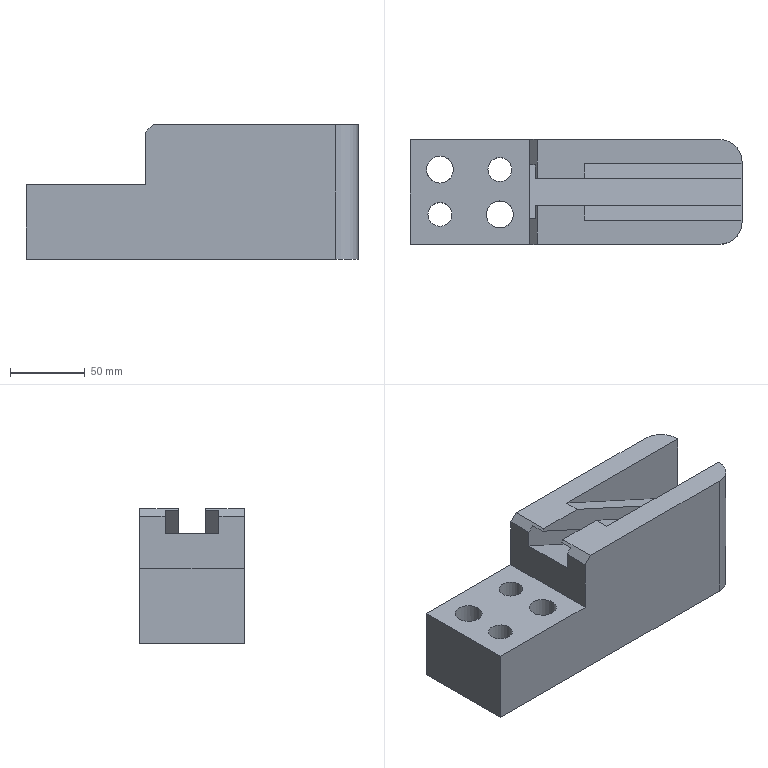Part | STEP file | solid 232 | 1 solid | 32 faces | box 221.793 x 70 x 90 mm | volume 892401 mm3 | plane 24 | cylinder 8 | commonest cylinder face diameters 16 x2 18 x2 26 x2 30 x2